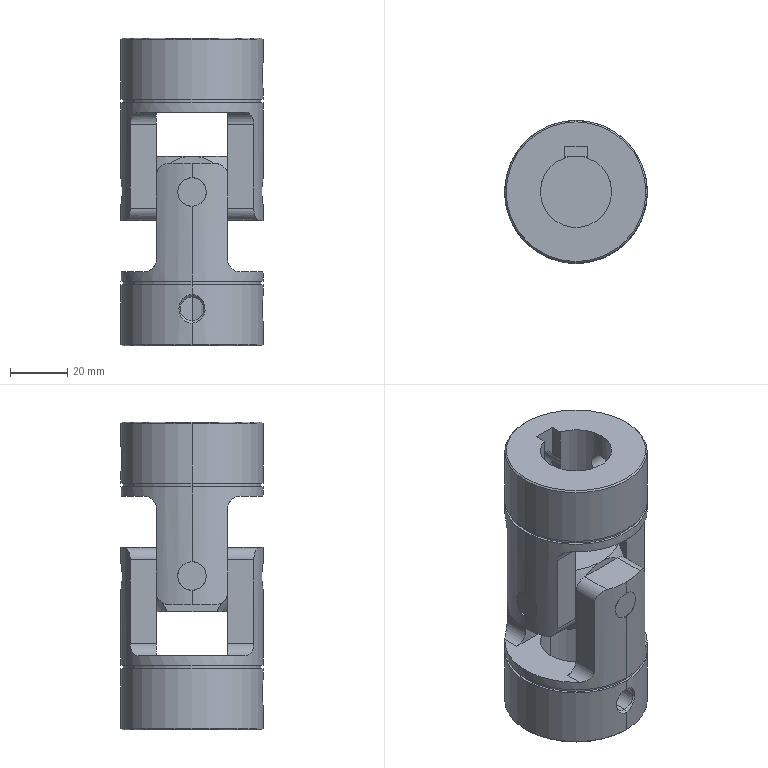Part | SolidWorks | 3 solids | 126 faces | box 50 x 50 x 108 mm | volume 130894 mm3 | cylinder 58 | plane 48 | cone 12 | sphere 8 | commonest cylinder face diameters 8.667 x16 10 x16 8.376 x8 50 x8 25 x6 48.267 x4